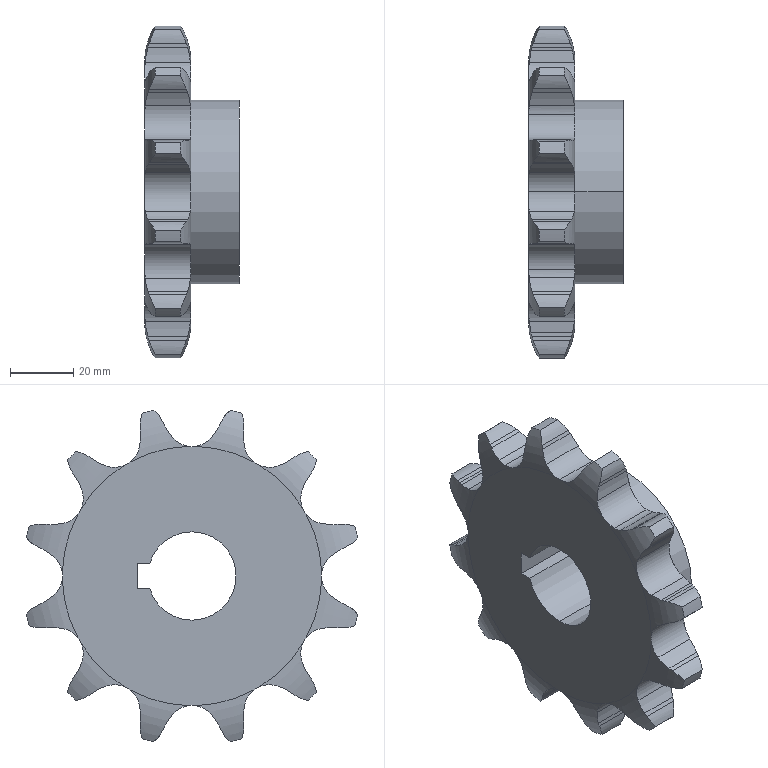Part | STEP file | 1 solid | 138 faces | box 30.002 x 105.245 x 105.245 mm | volume 117979 mm3 | cylinder 84 | plane 30 | torus 24 | commonest cylinder face diameters 23.691 x26 41.467 x26 16.059 x15 108 x12 28 x3 58.296 x2